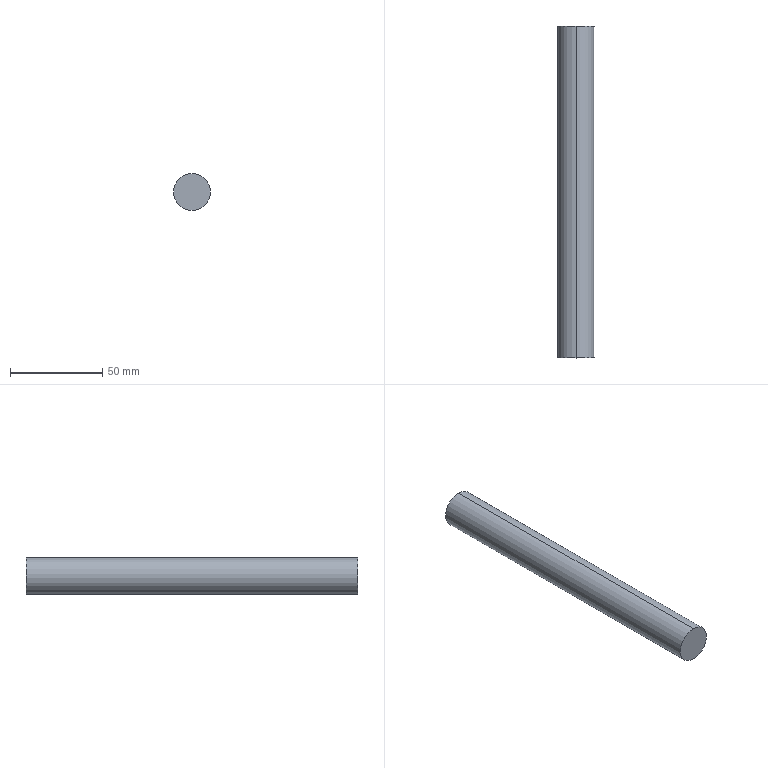Part | SolidWorks | features Extrusion 1 | 1 solid | 4 faces | box 20 x 180 x 20 mm | volume 56549 mm3 | cylinder 2 | plane 2 | commonest cylinder face diameters 20 x2
STEP:
#1=CARTESIAN_POINT('',(0.,180.,10.));
#2=VERTEX_POINT('',#1);
#3=CARTESIAN_POINT('',(0.,180.,-10.));
#4=VERTEX_POINT('',#3);
#5=CARTESIAN_POINT('',(0.,180.,0.));
#6=DIRECTION('',(0.,1.,0.));
#7=DIRECTION('',(0.,0.,1.));
#8=AXIS2_PLACEMENT_3D('',#5,#6,#7);
#9=CIRCLE('',#8,10.);
#10=EDGE_CURVE('',#2,#4,#9,.T.);
#11=ORIENTED_EDGE('',*,*,#10,.F.);
#12=CARTESIAN_POINT('',(0.,0.,10.));
#13=VERTEX_POINT('',#12);
#14=CARTESIAN_POINT('',(0.,180.,10.));
#15=DIRECTION('',(0.,-1.,0.));
#16=VECTOR('',#15,1000.);
#17=LINE('',#14,#16);
#18=EDGE_CURVE('',#2,#13,#17,.T.);
#19=ORIENTED_EDGE('',*,*,#18,.T.);
#20=CARTESIAN_POINT('',(0.,0.,-10.));
#21=VERTEX_POINT('',#20);
#22=CARTESIAN_POINT('',(0.,0.,0.));
#23=DIRECTION('',(0.,1.,0.));
#24=DIRECTION('',(0.,0.,1.));
#25=AXIS2_PLACEMENT_3D('',#22,#23,#24);
#26=CIRCLE('',#25,10.);
#27=EDGE_CURVE('',#13,#21,#26,.T.);
#28=ORIENTED_EDGE('',*,*,#27,.T.);
#29=CARTESIAN_POINT('',(0.,180.,-10.));
#30=DIRECTION('',(0.,-1.,0.));
#31=VECTOR('',#30,1000.);
#32=LINE('',#29,#31);
#33=EDGE_CURVE('',#4,#21,#32,.T.);
#34=ORIENTED_EDGE('',*,*,#33,.F.);
#35=EDGE_LOOP('',(#11,#19,#28,#34));
#36=FACE_OUTER_BOUND('',#35,.T.);
#37=CARTESIAN_POINT('',(0.,180.,0.));
#38=DIRECTION('',(0.,-1.,0.));
#39=DIRECTION('',(0.,0.,-1.));
#40=AXIS2_PLACEMENT_3D('',#37,#38,#39);
#41=CYLINDRICAL_SURFACE('',#40,10.);
#42=ADVANCED_FACE('',(#36),#41,.T.);
#43=ORIENTED_EDGE('',*,*,#18,.F.);
#44=CARTESIAN_POINT('',(0.,180.,0.));
#45=DIRECTION('',(0.,1.,0.));
#46=DIRECTION('',(0.,0.,1.));
#47=AXIS2_PLACEMENT_3D('',#44,#45,#46);
#48=CIRCLE('',#47,10.);
#49=EDGE_CURVE('',#4,#2,#48,.T.);
#50=ORIENTED_EDGE('',*,*,#49,.F.);
#51=ORIENTED_EDGE('',*,*,#33,.T.);
#52=CARTESIAN_POINT('',(0.,0.,0.));
#53=DIRECTION('',(0.,1.,0.));
#54=DIRECTION('',(0.,0.,1.));
#55=AXIS2_PLACEMENT_3D('',#52,#53,#54);
#56=CIRCLE('',#55,10.);
#57=EDGE_CURVE('',#21,#13,#56,.T.);
#58=ORIENTED_EDGE('',*,*,#57,.T.);
#59=EDGE_LOOP('',(#43,#50,#51,#58));
#60=FACE_OUTER_BOUND('',#59,.T.);
#61=CARTESIAN_POINT('',(0.,180.,0.));
#62=DIRECTION('',(0.,-1.,0.));
#63=DIRECTION('',(0.,0.,-1.));
#64=AXIS2_PLACEMENT_3D('',#61,#62,#63);
#65=CYLINDRICAL_SURFACE('',#64,10.);
#66=ADVANCED_FACE('',(#60),#65,.T.);
#67=ORIENTED_EDGE('',*,*,#49,.T.);
#68=ORIENTED_EDGE('',*,*,#10,.T.);
#69=EDGE_LOOP('',(#67,#68));
#70=FACE_OUTER_BOUND('',#69,.T.);
#71=CARTESIAN_POINT('',(0.,180.,0.));
#72=DIRECTION('',(0.,1.,0.));
#73=DIRECTION('',(0.,0.,1.));
#74=AXIS2_PLACEMENT_3D('',#71,#72,#73);
#75=PLANE('',#74);
#76=ADVANCED_FACE('',(#70),#75,.T.);
#77=ORIENTED_EDGE('',*,*,#57,.F.);
#78=ORIENTED_EDGE('',*,*,#27,.F.);
#79=EDGE_LOOP('',(#77,#78));
#80=FACE_OUTER_BOUND('',#79,.T.);
#81=CARTESIAN_POINT('',(0.,0.,0.));
#82=DIRECTION('',(0.,1.,0.));
#83=DIRECTION('',(0.,0.,1.));
#84=AXIS2_PLACEMENT_3D('',#81,#82,#83);
#85=PLANE('',#84);
#86=ADVANCED_FACE('',(#80),#85,.F.);
#87=CLOSED_SHELL('',(#42,#66,#76,#86));
#88=MANIFOLD_SOLID_BREP('',#87);
#89=CARTESIAN_POINT('',(0.,0.,0.));
#90=DIRECTION('',(0.,0.,1.));
#91=DIRECTION('',(1.,0.,0.));
#92=AXIS2_PLACEMENT_3D('',#89,#90,#91);
#93=(LENGTH_UNIT()NAMED_UNIT(*)SI_UNIT(.MILLI.,.METRE.));
#94=UNCERTAINTY_MEASURE_WITH_UNIT(LENGTH_MEASURE(0.00001),#93,'','');
#95=(NAMED_UNIT(*)PLANE_ANGLE_UNIT()SI_UNIT($,.RADIAN.));
#96=(NAMED_UNIT(*)SI_UNIT($,.STERADIAN.)SOLID_ANGLE_UNIT());
#97=(GEOMETRIC_REPRESENTATION_CONTEXT(3)GLOBAL_UNCERTAINTY_ASSIGNED_CONTEXT((#94))GLOBAL_UNIT_ASSIGNED_CONTEXT((#93,#95,#96))REPRESENTATION_CONTEXT('',''));
#98=ADVANCED_BREP_SHAPE_REPRESENTATION('',(#88,#92),#97);